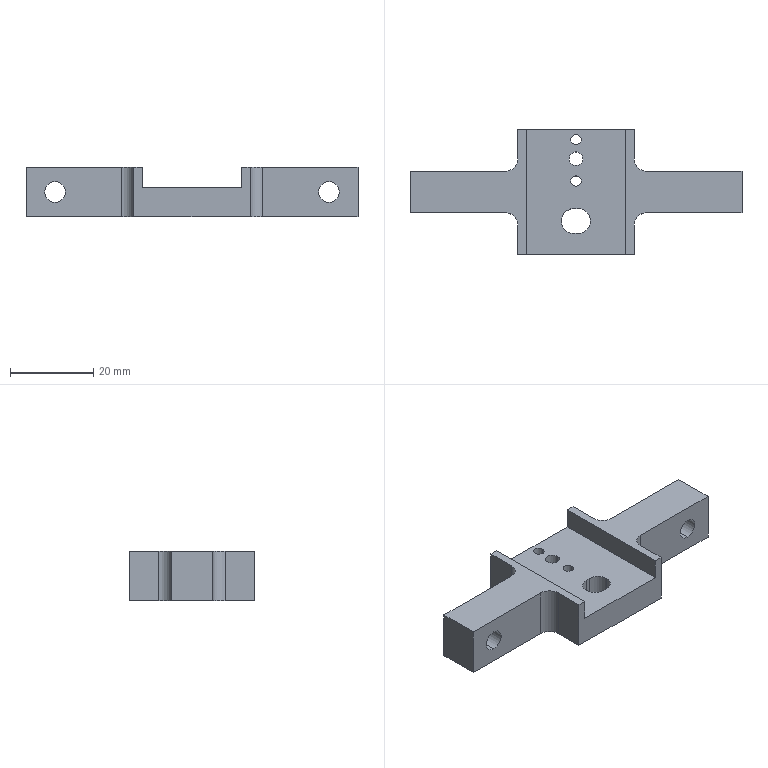Part | STEP file | 11-FG-E00611 | 1 solid | 53 faces | box 80 x 30 x 12 mm | volume 11899 mm3 | cylinder 25 | plane 20 | cone 8 | commonest cylinder face diameters 2.5 x12 6 x7 5 x4 3.3 x2